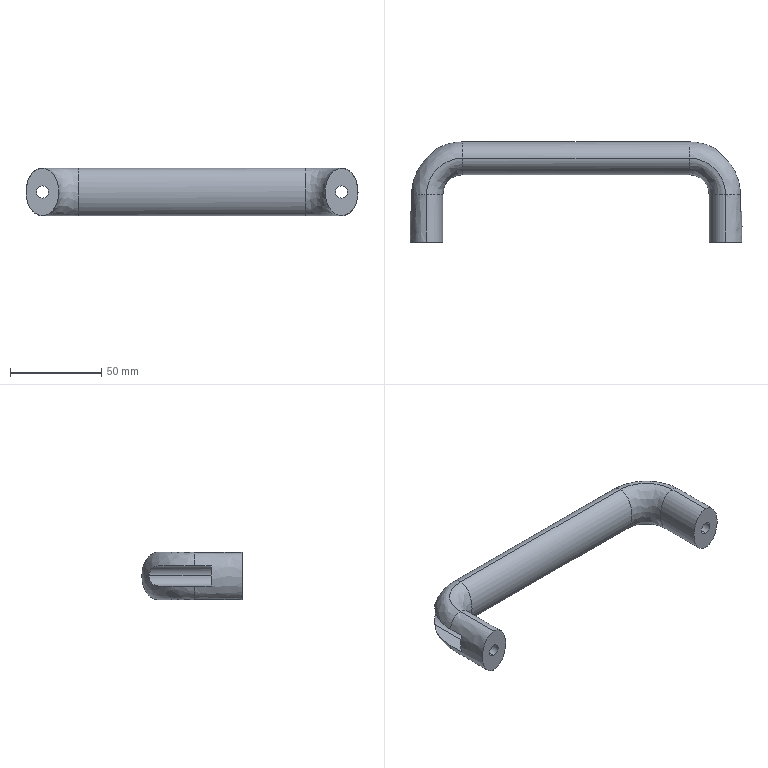Part | SolidWorks | features BaseBody 1 | 1 solid | 28 faces | box 182 x 55 x 26 mm | volume 78425 mm3 | plane 10 | spline 10 | cylinder 8 | commonest cylinder face diameters 6.6 x4 11 x4
STEP:
#1=CARTESIAN_POINT('',(76.5,51.115,0.));
#2=VERTEX_POINT('',#1);
#3=CARTESIAN_POINT('',(82.,45.817,-5.5));
#4=VERTEX_POINT('',#3);
#5=CARTESIAN_POINT('',(76.5,51.115,0.));
#6=CARTESIAN_POINT('',(76.5,51.115,-0.4392));
#7=CARTESIAN_POINT('',(76.552,51.067,-0.8654));
#8=CARTESIAN_POINT('',(76.701,50.931,-1.487));
#9=CARTESIAN_POINT('',(76.762,50.874,-1.691));
#10=CARTESIAN_POINT('',(76.904,50.743,-2.079));
#11=CARTESIAN_POINT('',(76.985,50.669,-2.266));
#12=CARTESIAN_POINT('',(77.163,50.504,-2.626));
#13=CARTESIAN_POINT('',(77.262,50.412,-2.8));
#14=CARTESIAN_POINT('',(77.471,50.217,-3.127));
#15=CARTESIAN_POINT('',(77.582,50.113,-3.281));
#16=CARTESIAN_POINT('',(77.814,49.895,-3.573));
#17=CARTESIAN_POINT('',(77.936,49.781,-3.71));
#18=CARTESIAN_POINT('',(78.188,49.543,-3.969));
#19=CARTESIAN_POINT('',(78.32,49.418,-4.091));
#20=CARTESIAN_POINT('',(78.993,48.778,-4.659));
#21=CARTESIAN_POINT('',(79.57,48.222,-4.975));
#22=CARTESIAN_POINT('',(80.778,47.04,-5.401));
#23=CARTESIAN_POINT('',(81.387,46.435,-5.5));
#24=CARTESIAN_POINT('',(82.,45.817,-5.5));
#25=B_SPLINE_CURVE_WITH_KNOTS('',3,(#5,#6,#7,#8,#9,#10,#11,#12,#13,#14,#15,#16,#17,#18,#19,#20,#21,#22,#23,#24),.UNSPECIFIED.,.F.,.F.,(4,2,2,2,2,2,2,2,2,4),(0.,0.001296,0.001943,0.002591,0.003239,0.003887,0.004535,0.005182,0.007774,0.01036),.UNSPECIFIED.);
#26=EDGE_CURVE('',#2,#4,#25,.T.);
#27=ORIENTED_EDGE('',*,*,#26,.F.);
#28=CARTESIAN_POINT('',(76.5,11.,0.));
#29=VERTEX_POINT('',#28);
#30=CARTESIAN_POINT('',(76.5,55.,0.));
#31=DIRECTION('',(0.,-1.,0.));
#32=VECTOR('',#31,1000.);
#33=LINE('',#30,#32);
#34=EDGE_CURVE('',#2,#29,#33,.T.);
#35=ORIENTED_EDGE('',*,*,#34,.T.);
#36=CARTESIAN_POINT('',(87.5,11.,0.));
#37=VERTEX_POINT('',#36);
#38=CARTESIAN_POINT('',(82.,11.,0.));
#39=DIRECTION('',(0.,1.,0.));
#40=DIRECTION('',(1.,0.,0.));
#41=AXIS2_PLACEMENT_3D('',#38,#39,#40);
#42=CIRCLE('',#41,5.5);
#43=EDGE_CURVE('',#37,#29,#42,.T.);
#44=ORIENTED_EDGE('',*,*,#43,.F.);
#45=CARTESIAN_POINT('',(87.5,17.,0.));
#46=VERTEX_POINT('',#45);
#47=CARTESIAN_POINT('',(87.5,55.,0.));
#48=DIRECTION('',(0.,-1.,0.));
#49=VECTOR('',#48,1000.);
#50=LINE('',#47,#49);
#51=EDGE_CURVE('',#46,#37,#50,.T.);
#52=ORIENTED_EDGE('',*,*,#51,.F.);
#53=CARTESIAN_POINT('',(82.,17.,-5.5));
#54=VERTEX_POINT('',#53);
#55=CARTESIAN_POINT('',(82.,17.,0.));
#56=DIRECTION('',(0.,-1.,0.));
#57=DIRECTION('',(1.,0.,0.));
#58=AXIS2_PLACEMENT_3D('',#55,#56,#57);
#59=CIRCLE('',#58,5.5);
#60=EDGE_CURVE('',#54,#46,#59,.T.);
#61=ORIENTED_EDGE('',*,*,#60,.F.);
#62=CARTESIAN_POINT('',(82.,55.,-5.5));
#63=DIRECTION('',(0.,-1.,0.));
#64=VECTOR('',#63,1000.);
#65=LINE('',#62,#64);
#66=EDGE_CURVE('',#4,#54,#65,.T.);
#67=ORIENTED_EDGE('',*,*,#66,.F.);
#68=EDGE_LOOP('',(#27,#35,#44,#52,#61,#67));
#69=FACE_OUTER_BOUND('',#68,.T.);
#70=CARTESIAN_POINT('',(82.,55.,0.));
#71=DIRECTION('',(0.,-1.,0.));
#72=DIRECTION('',(1.,0.,0.));
#73=AXIS2_PLACEMENT_3D('',#70,#71,#72);
#74=CYLINDRICAL_SURFACE('',#73,5.5);
#75=ADVANCED_FACE('',(#69),#74,.F.);
#76=CARTESIAN_POINT('',(-87.5,17.,0.));
#77=VERTEX_POINT('',#76);
#78=CARTESIAN_POINT('',(-82.,17.,-5.5));
#79=VERTEX_POINT('',#78);
#80=CARTESIAN_POINT('',(-82.,17.,0.));
#81=DIRECTION('',(0.,-1.,0.));
#82=DIRECTION('',(1.,0.,0.));
#83=AXIS2_PLACEMENT_3D('',#80,#81,#82);
#84=CIRCLE('',#83,5.5);
#85=EDGE_CURVE('',#77,#79,#84,.T.);
#86=ORIENTED_EDGE('',*,*,#85,.F.);
#87=CARTESIAN_POINT('',(-87.5,11.,0.));
#88=VERTEX_POINT('',#87);
#89=CARTESIAN_POINT('',(-87.5,55.,0.));
#90=DIRECTION('',(0.,-1.,0.));
#91=VECTOR('',#90,1000.);
#92=LINE('',#89,#91);
#93=EDGE_CURVE('',#77,#88,#92,.T.);
#94=ORIENTED_EDGE('',*,*,#93,.T.);
#95=CARTESIAN_POINT('',(-76.5,11.,0.));
#96=VERTEX_POINT('',#95);
#97=CARTESIAN_POINT('',(-82.,11.,0.));
#98=DIRECTION('',(0.,1.,0.));
#99=DIRECTION('',(1.,0.,0.));
#100=AXIS2_PLACEMENT_3D('',#97,#98,#99);
#101=CIRCLE('',#100,5.5);
#102=EDGE_CURVE('',#96,#88,#101,.T.);
#103=ORIENTED_EDGE('',*,*,#102,.F.);
#104=CARTESIAN_POINT('',(-76.5,51.115,0.));
#105=VERTEX_POINT('',#104);
#106=CARTESIAN_POINT('',(-76.5,55.,0.));
#107=DIRECTION('',(0.,-1.,0.));
#108=VECTOR('',#107,1000.);
#109=LINE('',#106,#108);
#110=EDGE_CURVE('',#105,#96,#109,.T.);
#111=ORIENTED_EDGE('',*,*,#110,.F.);
#112=CARTESIAN_POINT('',(-82.,45.817,-5.5));
#113=VERTEX_POINT('',#112);
#114=CARTESIAN_POINT('',(-82.,45.817,-5.5));
#115=CARTESIAN_POINT('',(-81.387,46.435,-5.5));
#116=CARTESIAN_POINT('',(-80.781,47.037,-5.4));
#117=CARTESIAN_POINT('',(-79.885,47.914,-5.087));
#118=CARTESIAN_POINT('',(-79.586,48.204,-4.953));
#119=CARTESIAN_POINT('',(-79.007,48.763,-4.626));
#120=CARTESIAN_POINT('',(-78.728,49.03,-4.435));
#121=CARTESIAN_POINT('',(-78.193,49.539,-3.985));
#122=CARTESIAN_POINT('',(-77.935,49.782,-3.723));
#123=CARTESIAN_POINT('',(-77.468,50.22,-3.139));
#124=CARTESIAN_POINT('',(-77.258,50.416,-2.815));
#125=CARTESIAN_POINT('',(-76.897,50.75,-2.09));
#126=CARTESIAN_POINT('',(-76.753,50.883,-1.703));
#127=CARTESIAN_POINT('',(-76.603,51.02,-1.082));
#128=CARTESIAN_POINT('',(-76.564,51.056,-0.8672));
#129=CARTESIAN_POINT('',(-76.513,51.103,-0.437));
#130=CARTESIAN_POINT('',(-76.5,51.115,-0.2197));
#131=CARTESIAN_POINT('',(-76.5,51.115,0.));
#132=B_SPLINE_CURVE_WITH_KNOTS('',3,(#114,#115,#116,#117,#118,#119,#120,#121,#122,#123,#124,#125,#126,#127,#128,#129,#130,#131),.UNSPECIFIED.,.F.,.F.,(4,2,2,2,2,2,2,2,4),(0.,0.002576,0.003865,0.005153,0.006441,0.007729,0.009018,0.009662,0.01031),.UNSPECIFIED.);
#133=EDGE_CURVE('',#113,#105,#132,.T.);
#134=ORIENTED_EDGE('',*,*,#133,.F.);
#135=CARTESIAN_POINT('',(-82.,55.,-5.5));
#136=DIRECTION('',(0.,1.,0.));
#137=VECTOR('',#136,1000.);
#138=LINE('',#135,#137);
#139=EDGE_CURVE('',#79,#113,#138,.T.);
#140=ORIENTED_EDGE('',*,*,#139,.F.);
#141=EDGE_LOOP('',(#86,#94,#103,#111,#134,#140));
#142=FACE_OUTER_BOUND('',#141,.T.);
#143=CARTESIAN_POINT('',(-82.,55.,0.));
#144=DIRECTION('',(0.,-1.,0.));
#145=DIRECTION('',(1.,0.,0.));
#146=AXIS2_PLACEMENT_3D('',#143,#144,#145);
#147=CYLINDRICAL_SURFACE('',#146,5.5);
#148=ADVANCED_FACE('',(#142),#147,.F.);
#149=CARTESIAN_POINT('',(82.,0.,-3.3));
#150=VERTEX_POINT('',#149);
#151=CARTESIAN_POINT('',(82.,0.,3.3));
#152=VERTEX_POINT('',#151);
#153=CARTESIAN_POINT('',(82.,0.,0.));
#154=DIRECTION('',(0.,1.,0.));
#155=DIRECTION('',(0.,0.,1.));
#156=AXIS2_PLACEMENT_3D('',#153,#154,#155);
#157=CIRCLE('',#156,3.3);
#158=EDGE_CURVE('',#150,#152,#157,.T.);
#159=ORIENTED_EDGE('',*,*,#158,.F.);
#160=CARTESIAN_POINT('',(82.,11.,-3.3));
#161=VERTEX_POINT('',#160);
#162=CARTESIAN_POINT('',(82.,17.,-3.3));
#163=DIRECTION('',(0.,1.,0.));
#164=VECTOR('',#163,1000.);
#165=LINE('',#162,#164);
#166=EDGE_CURVE('',#150,#161,#165,.T.);
#167=ORIENTED_EDGE('',*,*,#166,.T.);
#168=CARTESIAN_POINT('',(82.,11.,3.3));
#169=VERTEX_POINT('',#168);
#170=CARTESIAN_POINT('',(82.,11.,0.));
#171=DIRECTION('',(0.,1.,0.));
#172=DIRECTION('',(0.,0.,1.));
#173=AXIS2_PLACEMENT_3D('',#170,#171,#172);
#174=CIRCLE('',#173,3.3);
#175=EDGE_CURVE('',#161,#169,#174,.T.);
#176=ORIENTED_EDGE('',*,*,#175,.T.);
#177=CARTESIAN_POINT('',(82.,17.,3.3));
#178=DIRECTION('',(0.,1.,0.));
#179=VECTOR('',#178,1000.);
#180=LINE('',#177,#179);
#181=EDGE_CURVE('',#152,#169,#180,.T.);
#182=ORIENTED_EDGE('',*,*,#181,.F.);
#183=EDGE_LOOP('',(#159,#167,#176,#182));
#184=FACE_OUTER_BOUND('',#183,.T.);
#185=CARTESIAN_POINT('',(82.,17.,0.));
#186=DIRECTION('',(0.,1.,0.));
#187=DIRECTION('',(0.,0.,1.));
#188=AXIS2_PLACEMENT_3D('',#185,#186,#187);
#189=CYLINDRICAL_SURFACE('',#188,3.3);
#190=ADVANCED_FACE('',(#184),#189,.F.);
#191=CARTESIAN_POINT('',(-82.,0.,3.3));
#192=VERTEX_POINT('',#191);
#193=CARTESIAN_POINT('',(-82.,0.,-3.3));
#194=VERTEX_POINT('',#193);
#195=CARTESIAN_POINT('',(-82.,0.,0.));
#196=DIRECTION('',(0.,-1.,0.));
#197=DIRECTION('',(0.,0.,1.));
#198=AXIS2_PLACEMENT_3D('',#195,#196,#197);
#199=CIRCLE('',#198,3.3);
#200=EDGE_CURVE('',#192,#194,#199,.T.);
#201=ORIENTED_EDGE('',*,*,#200,.T.);
#202=CARTESIAN_POINT('',(-82.,11.,-3.3));
#203=VERTEX_POINT('',#202);
#204=CARTESIAN_POINT('',(-82.,17.,-3.3));
#205=DIRECTION('',(0.,1.,0.));
#206=VECTOR('',#205,1000.);
#207=LINE('',#204,#206);
#208=EDGE_CURVE('',#194,#203,#207,.T.);
#209=ORIENTED_EDGE('',*,*,#208,.T.);
#210=CARTESIAN_POINT('',(-82.,11.,3.3));
#211=VERTEX_POINT('',#210);
#212=CARTESIAN_POINT('',(-82.,11.,0.));
#213=DIRECTION('',(0.,1.,0.));
#214=DIRECTION('',(0.,0.,1.));
#215=AXIS2_PLACEMENT_3D('',#212,#213,#214);
#216=CIRCLE('',#215,3.3);
#217=EDGE_CURVE('',#203,#211,#216,.T.);
#218=ORIENTED_EDGE('',*,*,#217,.T.);
#219=CARTESIAN_POINT('',(-82.,17.,3.3));
#220=DIRECTION('',(0.,1.,0.));
#221=VECTOR('',#220,1000.);
#222=LINE('',#219,#221);
#223=EDGE_CURVE('',#192,#211,#222,.T.);
#224=ORIENTED_EDGE('',*,*,#223,.F.);
#225=EDGE_LOOP('',(#201,#209,#218,#224));
#226=FACE_OUTER_BOUND('',#225,.T.);
#227=CARTESIAN_POINT('',(-82.,17.,0.));
#228=DIRECTION('',(0.,1.,0.));
#229=DIRECTION('',(0.,0.,1.));
#230=AXIS2_PLACEMENT_3D('',#227,#228,#229);
#231=CYLINDRICAL_SURFACE('',#230,3.3);
#232=ADVANCED_FACE('',(#226),#231,.F.);
#233=ORIENTED_EDGE('',*,*,#200,.F.);
#234=CARTESIAN_POINT('',(-82.,0.,0.));
#235=DIRECTION('',(0.,-1.,0.));
#236=DIRECTION('',(0.,0.,1.));
#237=AXIS2_PLACEMENT_3D('',#234,#235,#236);
#238=CIRCLE('',#237,3.3);
#239=EDGE_CURVE('',#194,#192,#238,.T.);
#240=ORIENTED_EDGE('',*,*,#239,.F.);
#241=EDGE_LOOP('',(#233,#240));
#242=FACE_BOUND('',#241,.T.);
#243=CARTESIAN_POINT('',(-82.,0.,-13.));
#244=VERTEX_POINT('',#243);
#245=CARTESIAN_POINT('',(-82.,0.,13.));
#246=VERTEX_POINT('',#245);
#247=CARTESIAN_POINT('',(-82.,0.,-13.));
#248=CARTESIAN_POINT('',(-64.,0.,-13.));
#249=CARTESIAN_POINT('',(-64.,0.,13.));
#250=CARTESIAN_POINT('',(-82.,0.,13.));
#251=(BOUNDED_CURVE()B_SPLINE_CURVE(3,(#247,#248,#249,#250),.UNSPECIFIED.,.F.,.F.)B_SPLINE_CURVE_WITH_KNOTS((4,4),(0.,0.0348),.UNSPECIFIED.)CURVE()GEOMETRIC_REPRESENTATION_ITEM()RATIONAL_B_SPLINE_CURVE((1.,0.3333,0.3333,1.))REPRESENTATION_ITEM(''));
#252=EDGE_CURVE('',#244,#246,#251,.T.);
#253=ORIENTED_EDGE('',*,*,#252,.T.);
#254=CARTESIAN_POINT('',(-82.,0.,13.));
#255=CARTESIAN_POINT('',(-100.,0.,13.));
#256=CARTESIAN_POINT('',(-100.,0.,-13.));
#257=CARTESIAN_POINT('',(-82.,0.,-13.));
#258=(BOUNDED_CURVE()B_SPLINE_CURVE(3,(#254,#255,#256,#257),.UNSPECIFIED.,.F.,.T.)B_SPLINE_CURVE_WITH_KNOTS((4,4),(0.,0.0348),.UNSPECIFIED.)CURVE()GEOMETRIC_REPRESENTATION_ITEM()RATIONAL_B_SPLINE_CURVE((1.,0.3333,0.3333,1.))REPRESENTATION_ITEM(''));
#259=EDGE_CURVE('',#246,#244,#258,.T.);
#260=ORIENTED_EDGE('',*,*,#259,.T.);
#261=EDGE_LOOP('',(#253,#260));
#262=FACE_OUTER_BOUND('',#261,.T.);
#263=CARTESIAN_POINT('',(-82.,0.,0.));
#264=DIRECTION('',(0.,1.,0.));
#265=DIRECTION('',(1.,0.,0.));
#266=AXIS2_PLACEMENT_3D('',#263,#264,#265);
#267=PLANE('',#266);
#268=ADVANCED_FACE('',(#242,#262),#267,.F.);
#269=CARTESIAN_POINT('',(-82.,11.,0.));
#270=DIRECTION('',(0.,1.,0.));
#271=DIRECTION('',(0.,0.,1.));
#272=AXIS2_PLACEMENT_3D('',#269,#270,#271);
#273=CIRCLE('',#272,3.3);
#274=EDGE_CURVE('',#211,#203,#273,.T.);
#275=ORIENTED_EDGE('',*,*,#274,.F.);
#276=ORIENTED_EDGE('',*,*,#217,.F.);
#277=EDGE_LOOP('',(#275,#276));
#278=FACE_BOUND('',#277,.T.);
#279=ORIENTED_EDGE('',*,*,#102,.T.);
#280=CARTESIAN_POINT('',(-82.,11.,0.));
#281=DIRECTION('',(0.,1.,0.));
#282=DIRECTION('',(1.,0.,0.));
#283=AXIS2_PLACEMENT_3D('',#280,#281,#282);
#284=CIRCLE('',#283,5.5);
#285=EDGE_CURVE('',#88,#96,#284,.T.);
#286=ORIENTED_EDGE('',*,*,#285,.T.);
#287=EDGE_LOOP('',(#279,#286));
#288=FACE_OUTER_BOUND('',#287,.T.);
#289=CARTESIAN_POINT('',(-78.7,11.,0.));
#290=DIRECTION('',(0.,-1.,0.));
#291=DIRECTION('',(0.,0.,-1.));
#292=AXIS2_PLACEMENT_3D('',#289,#290,#291);
#293=PLANE('',#292);
#294=ADVANCED_FACE('',(#278,#288),#293,.F.);
#295=CARTESIAN_POINT('',(-90.155,17.,5.5));
#296=VERTEX_POINT('',#295);
#297=CARTESIAN_POINT('',(-82.,17.,5.5));
#298=VERTEX_POINT('',#297);
#299=CARTESIAN_POINT('',(-82.,17.,5.5));
#300=DIRECTION('',(1.,0.,0.));
#301=VECTOR('',#300,1000.);
#302=LINE('',#299,#301);
#303=EDGE_CURVE('',#296,#298,#302,.T.);
#304=ORIENTED_EDGE('',*,*,#303,.T.);
#305=CARTESIAN_POINT('',(-82.,17.,0.));
#306=DIRECTION('',(0.,-1.,0.));
#307=DIRECTION('',(1.,0.,0.));
#308=AXIS2_PLACEMENT_3D('',#305,#306,#307);
#309=CIRCLE('',#308,5.5);
#310=EDGE_CURVE('',#298,#77,#309,.T.);
#311=ORIENTED_EDGE('',*,*,#310,.T.);
#312=ORIENTED_EDGE('',*,*,#85,.T.);
#313=CARTESIAN_POINT('',(-90.155,17.,-5.5));
#314=VERTEX_POINT('',#313);
#315=CARTESIAN_POINT('',(-82.,17.,-5.5));
#316=DIRECTION('',(-1.,0.,0.));
#317=VECTOR('',#316,1000.);
#318=LINE('',#315,#317);
#319=EDGE_CURVE('',#79,#314,#318,.T.);
#320=ORIENTED_EDGE('',*,*,#319,.T.);
#321=CARTESIAN_POINT('',(-90.155,17.,-5.5));
#322=CARTESIAN_POINT('',(-91.301,17.,-1.956));
#323=CARTESIAN_POINT('',(-91.301,17.,1.956));
#324=CARTESIAN_POINT('',(-90.155,17.,5.5));
#325=(BOUNDED_CURVE()B_SPLINE_CURVE(3,(#321,#322,#323,#324),.UNSPECIFIED.,.F.,.T.)B_SPLINE_CURVE_WITH_KNOTS((4,4),(0.,0.01112),.UNSPECIFIED.)CURVE()GEOMETRIC_REPRESENTATION_ITEM()RATIONAL_B_SPLINE_CURVE((0.5246,0.4918,0.4918,0.5246))REPRESENTATION_ITEM(''));
#326=EDGE_CURVE('',#314,#296,#325,.T.);
#327=ORIENTED_EDGE('',*,*,#326,.T.);
#328=EDGE_LOOP('',(#304,#311,#312,#320,#327));
#329=FACE_OUTER_BOUND('',#328,.T.);
#330=CARTESIAN_POINT('',(-82.,17.,0.));
#331=DIRECTION('',(0.,-1.,0.));
#332=DIRECTION('',(-1.,0.,0.));
#333=AXIS2_PLACEMENT_3D('',#330,#331,#332);
#334=PLANE('',#333);
#335=ADVANCED_FACE('',(#329),#334,.F.);
#336=CARTESIAN_POINT('',(82.,11.,0.));
#337=DIRECTION('',(0.,1.,0.));
#338=DIRECTION('',(0.,0.,1.));
#339=AXIS2_PLACEMENT_3D('',#336,#337,#338);
#340=CIRCLE('',#339,3.3);
#341=EDGE_CURVE('',#169,#161,#340,.T.);
#342=ORIENTED_EDGE('',*,*,#341,.F.);
#343=ORIENTED_EDGE('',*,*,#175,.F.);
#344=EDGE_LOOP('',(#342,#343));
#345=FACE_BOUND('',#344,.T.);
#346=ORIENTED_EDGE('',*,*,#43,.T.);
#347=CARTESIAN_POINT('',(82.,11.,0.));
#348=DIRECTION('',(0.,1.,0.));
#349=DIRECTION('',(1.,0.,0.));
#350=AXIS2_PLACEMENT_3D('',#347,#348,#349);
#351=CIRCLE('',#350,5.5);
#352=EDGE_CURVE('',#29,#37,#351,.T.);
#353=ORIENTED_EDGE('',*,*,#352,.T.);
#354=EDGE_LOOP('',(#346,#353));
#355=FACE_OUTER_BOUND('',#354,.T.);
#356=CARTESIAN_POINT('',(85.3,11.,0.));
#357=DIRECTION('',(0.,-1.,0.));
#358=DIRECTION('',(0.,0.,-1.));
#359=AXIS2_PLACEMENT_3D('',#356,#357,#358);
#360=PLANE('',#359);
#361=ADVANCED_FACE('',(#345,#355),#360,.F.);
#362=CARTESIAN_POINT('',(82.,0.,0.));
#363=DIRECTION('',(0.,1.,0.));
#364=DIRECTION('',(0.,0.,1.));
#365=AXIS2_PLACEMENT_3D('',#362,#363,#364);
#366=CIRCLE('',#365,3.3);
#367=EDGE_CURVE('',#152,#150,#366,.T.);
#368=ORIENTED_EDGE('',*,*,#367,.T.);
#369=ORIENTED_EDGE('',*,*,#158,.T.);
#370=EDGE_LOOP('',(#368,#369));
#371=FACE_BOUND('',#370,.T.);
#372=CARTESIAN_POINT('',(82.,0.,13.));
#373=VERTEX_POINT('',#372);
#374=CARTESIAN_POINT('',(82.,0.,-13.));
#375=VERTEX_POINT('',#374);
#376=CARTESIAN_POINT('',(82.,0.,13.));
#377=CARTESIAN_POINT('',(100.,0.,13.));
#378=CARTESIAN_POINT('',(100.,0.,-13.));
#379=CARTESIAN_POINT('',(82.,0.,-13.));
#380=(BOUNDED_CURVE()B_SPLINE_CURVE(3,(#376,#377,#378,#379),.UNSPECIFIED.,.F.,.F.)B_SPLINE_CURVE_WITH_KNOTS((4,4),(0.,0.0348),.UNSPECIFIED.)CURVE()GEOMETRIC_REPRESENTATION_ITEM()RATIONAL_B_SPLINE_CURVE((1.,0.3333,0.3333,1.))REPRESENTATION_ITEM(''));
#381=EDGE_CURVE('',#373,#375,#380,.T.);
#382=ORIENTED_EDGE('',*,*,#381,.F.);
#383=CARTESIAN_POINT('',(82.,0.,-13.));
#384=CARTESIAN_POINT('',(64.,0.,-13.));
#385=CARTESIAN_POINT('',(64.,0.,13.));
#386=CARTESIAN_POINT('',(82.,0.,13.));
#387=(BOUNDED_CURVE()B_SPLINE_CURVE(3,(#383,#384,#385,#386),.UNSPECIFIED.,.F.,.T.)B_SPLINE_CURVE_WITH_KNOTS((4,4),(0.,0.0348),.UNSPECIFIED.)CURVE()GEOMETRIC_REPRESENTATION_ITEM()RATIONAL_B_SPLINE_CURVE((1.,0.3333,0.3333,1.))REPRESENTATION_ITEM(''));
#388=EDGE_CURVE('',#375,#373,#387,.T.);
#389=ORIENTED_EDGE('',*,*,#388,.F.);
#390=EDGE_LOOP('',(#382,#389));
#391=FACE_OUTER_BOUND('',#390,.T.);
#392=CARTESIAN_POINT('',(82.,0.,0.));
#393=DIRECTION('',(0.,-1.,0.));
#394=DIRECTION('',(-1.,0.,0.));
#395=AXIS2_PLACEMENT_3D('',#392,#393,#394);
#396=PLANE('',#395);
#397=ADVANCED_FACE('',(#371,#391),#396,.T.);
#398=ORIENTED_EDGE('',*,*,#60,.T.);
#399=CARTESIAN_POINT('',(82.,17.,5.5));
#400=VERTEX_POINT('',#399);
#401=CARTESIAN_POINT('',(82.,17.,0.));
#402=DIRECTION('',(0.,-1.,0.));
#403=DIRECTION('',(1.,0.,0.));
#404=AXIS2_PLACEMENT_3D('',#401,#402,#403);
#405=CIRCLE('',#404,5.5);
#406=EDGE_CURVE('',#46,#400,#405,.T.);
#407=ORIENTED_EDGE('',*,*,#406,.T.);
#408=CARTESIAN_POINT('',(90.155,17.,5.5));
#409=VERTEX_POINT('',#408);
#410=CARTESIAN_POINT('',(82.,17.,5.5));
#411=DIRECTION('',(-1.,0.,0.));
#412=VECTOR('',#411,1000.);
#413=LINE('',#410,#412);
#414=EDGE_CURVE('',#409,#400,#413,.T.);
#415=ORIENTED_EDGE('',*,*,#414,.F.);
#416=CARTESIAN_POINT('',(90.155,17.,-5.5));
#417=VERTEX_POINT('',#416);
#418=CARTESIAN_POINT('',(90.155,17.,-5.5));
#419=CARTESIAN_POINT('',(91.301,17.,-1.956));
#420=CARTESIAN_POINT('',(91.301,17.,1.956));
#421=CARTESIAN_POINT('',(90.155,17.,5.5));
#422=(BOUNDED_CURVE()B_SPLINE_CURVE(3,(#418,#419,#420,#421),.UNSPECIFIED.,.F.,.F.)B_SPLINE_CURVE_WITH_KNOTS((4,4),(0.,0.01112),.UNSPECIFIED.)CURVE()GEOMETRIC_REPRESENTATION_ITEM()RATIONAL_B_SPLINE_CURVE((0.5246,0.4918,0.4918,0.5246))REPRESENTATION_ITEM(''));
#423=EDGE_CURVE('',#417,#409,#422,.T.);
#424=ORIENTED_EDGE('',*,*,#423,.F.);
#425=CARTESIAN_POINT('',(82.,17.,-5.5));
#426=DIRECTION('',(1.,0.,0.));
#427=VECTOR('',#426,1000.);
#428=LINE('',#425,#427);
#429=EDGE_CURVE('',#54,#417,#428,.T.);
#430=ORIENTED_EDGE('',*,*,#429,.F.);
#431=EDGE_LOOP('',(#398,#407,#415,#424,#430));
#432=FACE_OUTER_BOUND('',#431,.T.);
#433=CARTESIAN_POINT('',(82.,17.,0.));
#434=DIRECTION('',(0.,-1.,0.));
#435=DIRECTION('',(0.,0.,-1.));
#436=AXIS2_PLACEMENT_3D('',#433,#434,#435);
#437=PLANE('',#436);
#438=ADVANCED_FACE('',(#432),#437,.F.);
#439=CARTESIAN_POINT('',(-82.,26.,13.));
#440=VERTEX_POINT('',#439);
#441=CARTESIAN_POINT('',(-82.,13.,13.));
#442=DIRECTION('',(0.,-1.,0.));
#443=VECTOR('',#442,1000.);
#444=LINE('',#441,#443);
#445=EDGE_CURVE('',#440,#246,#444,.T.);
#446=ORIENTED_EDGE('',*,*,#445,.T.);
#447=ORIENTED_EDGE('',*,*,#252,.F.);
#448=CARTESIAN_POINT('',(-82.,26.,-13.));
#449=VERTEX_POINT('',#448);
#450=CARTESIAN_POINT('',(-82.,13.,-13.));
#451=DIRECTION('',(0.,1.,0.));
#452=VECTOR('',#451,1000.);
#453=LINE('',#450,#452);
#454=EDGE_CURVE('',#244,#449,#453,.T.);
#455=ORIENTED_EDGE('',*,*,#454,.T.);
#456=CARTESIAN_POINT('',(-82.,26.,13.));
#457=CARTESIAN_POINT('',(-64.,26.,13.));
#458=CARTESIAN_POINT('',(-64.,26.,-13.));
#459=CARTESIAN_POINT('',(-82.,26.,-13.));
#460=(BOUNDED_CURVE()B_SPLINE_CURVE(3,(#456,#457,#458,#459),.UNSPECIFIED.,.F.,.F.)B_SPLINE_CURVE_WITH_KNOTS((4,4),(0.,1.),.UNSPECIFIED.)CURVE()GEOMETRIC_REPRESENTATION_ITEM()RATIONAL_B_SPLINE_CURVE((1.,0.3333,0.3333,1.))REPRESENTATION_ITEM(''));
#461=EDGE_CURVE('',#440,#449,#460,.T.);
#462=ORIENTED_EDGE('',*,*,#461,.F.);
#463=EDGE_LOOP('',(#446,#447,#455,#462));
#464=FACE_OUTER_BOUND('',#463,.T.);
#465=CARTESIAN_POINT('',(-82.,26.,13.));
#466=CARTESIAN_POINT('',(-82.,0.,13.));
#467=CARTESIAN_POINT('',(-64.,26.,13.));
#468=CARTESIAN_POINT('',(-64.,0.,13.));
#469=CARTESIAN_POINT('',(-64.,26.,-13.));
#470=CARTESIAN_POINT('',(-64.,0.,-13.));
#471=CARTESIAN_POINT('',(-82.,26.,-13.));
#472=CARTESIAN_POINT('',(-82.,0.,-13.));
#473=(BOUNDED_SURFACE()B_SPLINE_SURFACE(3,1,((#465,#466),(#467,#468),(#469,#470),(#471,#472)),.UNSPECIFIED.,.F.,.F.,.T.)B_SPLINE_SURFACE_WITH_KNOTS((4,4),(2,2),(0.,1.),(0.,1.),.UNSPECIFIED.)GEOMETRIC_REPRESENTATION_ITEM()RATIONAL_B_SPLINE_SURFACE(((1.,1.),(0.3333,0.3333),(0.3333,0.3333),(1.,1.)))REPRESENTATION_ITEM('')SURFACE());
#474=ADVANCED_FACE('',(#464),#473,.F.);
#475=CARTESIAN_POINT('',(82.,26.,-13.));
#476=VERTEX_POINT('',#475);
#477=CARTESIAN_POINT('',(82.,13.,-13.));
#478=DIRECTION('',(0.,1.,0.));
#479=VECTOR('',#478,1000.);
#480=LINE('',#477,#479);
#481=EDGE_CURVE('',#375,#476,#480,.T.);
#482=ORIENTED_EDGE('',*,*,#481,.F.);
#483=ORIENTED_EDGE('',*,*,#388,.T.);
#484=CARTESIAN_POINT('',(82.,26.,13.));
#485=VERTEX_POINT('',#484);
#486=CARTESIAN_POINT('',(82.,13.,13.));
#487=DIRECTION('',(0.,-1.,0.));
#488=VECTOR('',#487,1000.);
#489=LINE('',#486,#488);
#490=EDGE_CURVE('',#485,#373,#489,.T.);
#491=ORIENTED_EDGE('',*,*,#490,.F.);
#492=CARTESIAN_POINT('',(82.,26.,-13.));
#493=CARTESIAN_POINT('',(64.,26.,-13.));
#494=CARTESIAN_POINT('',(64.,26.,13.));
#495=CARTESIAN_POINT('',(82.,26.,13.));
#496=(BOUNDED_CURVE()B_SPLINE_CURVE(3,(#492,#493,#494,#495),.UNSPECIFIED.,.F.,.T.)B_SPLINE_CURVE_WITH_KNOTS((4,4),(0.,1.),.UNSPECIFIED.)CURVE()GEOMETRIC_REPRESENTATION_ITEM()RATIONAL_B_SPLINE_CURVE((1.,0.3333,0.3333,1.))REPRESENTATION_ITEM(''));
#497=EDGE_CURVE('',#476,#485,#496,.T.);
#498=ORIENTED_EDGE('',*,*,#497,.F.);
#499=EDGE_LOOP('',(#482,#483,#491,#498));
#500=FACE_OUTER_BOUND('',#499,.T.);
#501=CARTESIAN_POINT('',(82.,26.,13.));
#502=CARTESIAN_POINT('',(82.,0.,13.));
#503=CARTESIAN_POINT('',(64.,26.,13.));
#504=CARTESIAN_POINT('',(64.,0.,13.));
#505=CARTESIAN_POINT('',(64.,26.,-13.));
#506=CARTESIAN_POINT('',(64.,0.,-13.));
#507=CARTESIAN_POINT('',(82.,26.,-13.));
#508=CARTESIAN_POINT('',(82.,0.,-13.));
#509=(BOUNDED_SURFACE()B_SPLINE_SURFACE(3,1,((#501,#502),(#503,#504),(#505,#506),(#507,#508)),.UNSPECIFIED.,.F.,.F.,.T.)B_SPLINE_SURFACE_WITH_KNOTS((4,4),(2,2),(0.,1.),(0.,1.),.UNSPECIFIED.)GEOMETRIC_REPRESENTATION_ITEM()RATIONAL_B_SPLINE_SURFACE(((1.,1.),(0.3333,0.3333),(0.3333,0.3333),(1.,1.)))REPRESENTATION_ITEM('')SURFACE());
#510=ADVANCED_FACE('',(#500),#509,.T.);
#511=CARTESIAN_POINT('',(-90.155,26.,5.5));
#512=VERTEX_POINT('',#511);
#513=CARTESIAN_POINT('',(-90.155,26.,5.5));
#514=CARTESIAN_POINT('',(-88.459,26.,10.747));
#515=CARTESIAN_POINT('',(-85.151,26.,13.));
#516=CARTESIAN_POINT('',(-82.,26.,13.));
#517=(BOUNDED_CURVE()B_SPLINE_CURVE(3,(#513,#514,#515,#516),.UNSPECIFIED.,.F.,.F.)B_SPLINE_CURVE_WITH_KNOTS((4,4),(0.611,1.),.UNSPECIFIED.)CURVE()GEOMETRIC_REPRESENTATION_ITEM()RATIONAL_B_SPLINE_CURVE((0.5246,0.5822,0.7407,1.))REPRESENTATION_ITEM(''));
#518=EDGE_CURVE('',#512,#440,#517,.T.);
#519=ORIENTED_EDGE('',*,*,#518,.F.);
#520=CARTESIAN_POINT('',(-90.155,55.,5.5));
#521=DIRECTION('',(0.,-1.,0.));
#522=VECTOR('',#521,1000.);
#523=LINE('',#520,#522);
#524=EDGE_CURVE('',#512,#296,#523,.T.);
#525=ORIENTED_EDGE('',*,*,#524,.T.);
#526=ORIENTED_EDGE('',*,*,#326,.F.);
#527=CARTESIAN_POINT('',(-90.155,26.,-5.5));
#528=VERTEX_POINT('',#527);
#529=CARTESIAN_POINT('',(-90.155,55.,-5.5));
#530=DIRECTION('',(0.,1.,0.));
#531=VECTOR('',#530,1000.);
#532=LINE('',#529,#531);
#533=EDGE_CURVE('',#314,#528,#532,.T.);
#534=ORIENTED_EDGE('',*,*,#533,.T.);
#535=CARTESIAN_POINT('',(-82.,26.,-13.));
#536=CARTESIAN_POINT('',(-85.151,26.,-13.));
#537=CARTESIAN_POINT('',(-88.459,26.,-10.747));
#538=CARTESIAN_POINT('',(-90.155,26.,-5.5));
#539=(BOUNDED_CURVE()B_SPLINE_CURVE(3,(#535,#536,#537,#538),.UNSPECIFIED.,.F.,.T.)B_SPLINE_CURVE_WITH_KNOTS((4,4),(0.,0.389),.UNSPECIFIED.)CURVE()GEOMETRIC_REPRESENTATION_ITEM()RATIONAL_B_SPLINE_CURVE((1.,0.7407,0.5822,0.5246))REPRESENTATION_ITEM(''));
#540=EDGE_CURVE('',#449,#528,#539,.T.);
#541=ORIENTED_EDGE('',*,*,#540,.F.);
#542=ORIENTED_EDGE('',*,*,#454,.F.);
#543=ORIENTED_EDGE('',*,*,#259,.F.);
#544=ORIENTED_EDGE('',*,*,#445,.F.);
#545=EDGE_LOOP('',(#519,#525,#526,#534,#541,#542,#543,#544));
#546=FACE_OUTER_BOUND('',#545,.T.);
#547=CARTESIAN_POINT('',(-82.,26.,-13.));
#548=CARTESIAN_POINT('',(-82.,0.,-13.));
#549=CARTESIAN_POINT('',(-100.,26.,-13.));
#550=CARTESIAN_POINT('',(-100.,0.,-13.));
#551=CARTESIAN_POINT('',(-100.,26.,13.));
#552=CARTESIAN_POINT('',(-100.,0.,13.));
#553=CARTESIAN_POINT('',(-82.,26.,13.));
#554=CARTESIAN_POINT('',(-82.,0.,13.));
#555=(BOUNDED_SURFACE()B_SPLINE_SURFACE(3,1,((#547,#548),(#549,#550),(#551,#552),(#553,#554)),.UNSPECIFIED.,.F.,.F.,.T.)B_SPLINE_SURFACE_WITH_KNOTS((4,4),(2,2),(0.,1.),(0.,1.),.UNSPECIFIED.)GEOMETRIC_REPRESENTATION_ITEM()RATIONAL_B_SPLINE_SURFACE(((1.,1.),(0.3333,0.3333),(0.3333,0.3333),(1.,1.)))REPRESENTATION_ITEM('')SURFACE());
#556=ADVANCED_FACE('',(#546),#555,.F.);
#557=ORIENTED_EDGE('',*,*,#533,.F.);
#558=ORIENTED_EDGE('',*,*,#319,.F.);
#559=ORIENTED_EDGE('',*,*,#139,.T.);
#560=CARTESIAN_POINT('',(-90.155,26.,-5.5));
#561=CARTESIAN_POINT('',(-90.155,33.309,-5.5));
#562=CARTESIAN_POINT('',(-87.438,40.328,-5.5));
#563=CARTESIAN_POINT('',(-82.,45.817,-5.5));
#564=(BOUNDED_CURVE()B_SPLINE_CURVE(3,(#560,#561,#562,#563),.UNSPECIFIED.,.F.,.F.)B_SPLINE_CURVE_WITH_KNOTS((4,4),(0.,0.02185),.UNSPECIFIED.)CURVE()GEOMETRIC_REPRESENTATION_ITEM()RATIONAL_B_SPLINE_CURVE((0.5246,0.4737,0.4481,0.4478))REPRESENTATION_ITEM(''));
#565=EDGE_CURVE('',#528,#113,#564,.T.);
#566=ORIENTED_EDGE('',*,*,#565,.F.);
#567=EDGE_LOOP('',(#557,#558,#559,#566));
#568=FACE_OUTER_BOUND('',#567,.T.);
#569=CARTESIAN_POINT('',(-82.,55.,-5.5));
#570=DIRECTION('',(0.,0.,-1.));
#571=DIRECTION('',(0.,-1.,0.));
#572=AXIS2_PLACEMENT_3D('',#569,#570,#571);
#573=PLANE('',#572);
#574=ADVANCED_FACE('',(#568),#573,.F.);
#575=CARTESIAN_POINT('',(-82.,45.817,5.5));
#576=VERTEX_POINT('',#575);
#577=CARTESIAN_POINT('',(-82.,55.,5.5));
#578=DIRECTION('',(0.,1.,0.));
#579=VECTOR('',#578,1000.);
#580=LINE('',#577,#579);
#581=EDGE_CURVE('',#298,#576,#580,.T.);
#582=ORIENTED_EDGE('',*,*,#581,.F.);
#583=ORIENTED_EDGE('',*,*,#303,.F.);
#584=ORIENTED_EDGE('',*,*,#524,.F.);
#585=CARTESIAN_POINT('',(-82.,45.817,5.5));
#586=CARTESIAN_POINT('',(-87.438,40.328,5.5));
#587=CARTESIAN_POINT('',(-90.155,33.309,5.5));
#588=CARTESIAN_POINT('',(-90.155,26.,5.5));
#589=(BOUNDED_CURVE()B_SPLINE_CURVE(3,(#585,#586,#587,#588),.UNSPECIFIED.,.F.,.F.)B_SPLINE_CURVE_WITH_KNOTS((4,4),(0.,0.02185),.UNSPECIFIED.)CURVE()GEOMETRIC_REPRESENTATION_ITEM()RATIONAL_B_SPLINE_CURVE((0.4478,0.4481,0.4737,0.5246))REPRESENTATION_ITEM(''));
#590=EDGE_CURVE('',#576,#512,#589,.T.);
#591=ORIENTED_EDGE('',*,*,#590,.F.);
#592=EDGE_LOOP('',(#582,#583,#584,#591));
#593=FACE_OUTER_BOUND('',#592,.T.);
#594=CARTESIAN_POINT('',(-82.,55.,5.5));
#595=DIRECTION('',(0.,0.,1.));
#596=DIRECTION('',(1.,0.,0.));
#597=AXIS2_PLACEMENT_3D('',#594,#595,#596);
#598=PLANE('',#597);
#599=ADVANCED_FACE('',(#593),#598,.F.);
#600=CARTESIAN_POINT('',(90.155,26.,5.5));
#601=VERTEX_POINT('',#600);
#602=CARTESIAN_POINT('',(82.,45.817,5.5));
#603=VERTEX_POINT('',#602);
#604=CARTESIAN_POINT('',(90.155,26.,5.5));
#605=CARTESIAN_POINT('',(90.155,33.309,5.5));
#606=CARTESIAN_POINT('',(87.438,40.328,5.5));
#607=CARTESIAN_POINT('',(82.,45.817,5.5));
#608=(BOUNDED_CURVE()B_SPLINE_CURVE(3,(#604,#605,#606,#607),.UNSPECIFIED.,.F.,.F.)B_SPLINE_CURVE_WITH_KNOTS((4,4),(0.,0.02185),.UNSPECIFIED.)CURVE()GEOMETRIC_REPRESENTATION_ITEM()RATIONAL_B_SPLINE_CURVE((0.5246,0.4737,0.4481,0.4478))REPRESENTATION_ITEM(''));
#609=EDGE_CURVE('',#601,#603,#608,.T.);
#610=ORIENTED_EDGE('',*,*,#609,.F.);
#611=CARTESIAN_POINT('',(90.155,13.,5.5));
#612=DIRECTION('',(0.,1.,0.));
#613=VECTOR('',#612,1000.);
#614=LINE('',#611,#613);
#615=EDGE_CURVE('',#409,#601,#614,.T.);
#616=ORIENTED_EDGE('',*,*,#615,.F.);
#617=ORIENTED_EDGE('',*,*,#414,.T.);
#618=CARTESIAN_POINT('',(82.,55.,5.5));
#619=DIRECTION('',(0.,1.,0.));
#620=VECTOR('',#619,1000.);
#621=LINE('',#618,#620);
#622=EDGE_CURVE('',#400,#603,#621,.T.);
#623=ORIENTED_EDGE('',*,*,#622,.T.);
#624=EDGE_LOOP('',(#610,#616,#617,#623));
#625=FACE_OUTER_BOUND('',#624,.T.);
#626=CARTESIAN_POINT('',(82.,55.,5.5));
#627=DIRECTION('',(0.,0.,-1.));
#628=DIRECTION('',(0.,-1.,0.));
#629=AXIS2_PLACEMENT_3D('',#626,#627,#628);
#630=PLANE('',#629);
#631=ADVANCED_FACE('',(#625),#630,.T.);
#632=ORIENTED_EDGE('',*,*,#429,.T.);
#633=CARTESIAN_POINT('',(90.155,26.,-5.5));
#634=VERTEX_POINT('',#633);
#635=CARTESIAN_POINT('',(90.155,13.,-5.5));
#636=DIRECTION('',(0.,-1.,0.));
#637=VECTOR('',#636,1000.);
#638=LINE('',#635,#637);
#639=EDGE_CURVE('',#634,#417,#638,.T.);
#640=ORIENTED_EDGE('',*,*,#639,.F.);
#641=CARTESIAN_POINT('',(82.,45.817,-5.5));
#642=CARTESIAN_POINT('',(87.438,40.328,-5.5));
#643=CARTESIAN_POINT('',(90.155,33.309,-5.5));
#644=CARTESIAN_POINT('',(90.155,26.,-5.5));
#645=(BOUNDED_CURVE()B_SPLINE_CURVE(3,(#641,#642,#643,#644),.UNSPECIFIED.,.F.,.F.)B_SPLINE_CURVE_WITH_KNOTS((4,4),(0.,0.02185),.UNSPECIFIED.)CURVE()GEOMETRIC_REPRESENTATION_ITEM()RATIONAL_B_SPLINE_CURVE((0.4478,0.4481,0.4737,0.5246))REPRESENTATION_ITEM(''));
#646=EDGE_CURVE('',#4,#634,#645,.T.);
#647=ORIENTED_EDGE('',*,*,#646,.F.);
#648=ORIENTED_EDGE('',*,*,#66,.T.);
#649=EDGE_LOOP('',(#632,#640,#647,#648));
#650=FACE_OUTER_BOUND('',#649,.T.);
#651=CARTESIAN_POINT('',(82.,55.,-5.5));
#652=DIRECTION('',(0.,0.,1.));
#653=DIRECTION('',(1.,0.,0.));
#654=AXIS2_PLACEMENT_3D('',#651,#652,#653);
#655=PLANE('',#654);
#656=ADVANCED_FACE('',(#650),#655,.T.);
#657=ORIENTED_EDGE('',*,*,#423,.T.);
#658=ORIENTED_EDGE('',*,*,#615,.T.);
#659=CARTESIAN_POINT('',(82.,26.,13.));
#660=CARTESIAN_POINT('',(85.151,26.,13.));
#661=CARTESIAN_POINT('',(88.459,26.,10.747));
#662=CARTESIAN_POINT('',(90.155,26.,5.5));
#663=(BOUNDED_CURVE()B_SPLINE_CURVE(3,(#659,#660,#661,#662),.UNSPECIFIED.,.F.,.F.)B_SPLINE_CURVE_WITH_KNOTS((4,4),(0.,0.389),.UNSPECIFIED.)CURVE()GEOMETRIC_REPRESENTATION_ITEM()RATIONAL_B_SPLINE_CURVE((1.,0.7407,0.5822,0.5246))REPRESENTATION_ITEM(''));
#664=EDGE_CURVE('',#485,#601,#663,.T.);
#665=ORIENTED_EDGE('',*,*,#664,.F.);
#666=ORIENTED_EDGE('',*,*,#490,.T.);
#667=ORIENTED_EDGE('',*,*,#381,.T.);
#668=ORIENTED_EDGE('',*,*,#481,.T.);
#669=CARTESIAN_POINT('',(90.155,26.,-5.5));
#670=CARTESIAN_POINT('',(88.459,26.,-10.747));
#671=CARTESIAN_POINT('',(85.151,26.,-13.));
#672=CARTESIAN_POINT('',(82.,26.,-13.));
#673=(BOUNDED_CURVE()B_SPLINE_CURVE(3,(#669,#670,#671,#672),.UNSPECIFIED.,.F.,.F.)B_SPLINE_CURVE_WITH_KNOTS((4,4),(0.611,1.),.UNSPECIFIED.)CURVE()GEOMETRIC_REPRESENTATION_ITEM()RATIONAL_B_SPLINE_CURVE((0.5246,0.5822,0.7407,1.))REPRESENTATION_ITEM(''));
#674=EDGE_CURVE('',#634,#476,#673,.T.);
#675=ORIENTED_EDGE('',*,*,#674,.F.);
#676=ORIENTED_EDGE('',*,*,#639,.T.);
#677=EDGE_LOOP('',(#657,#658,#665,#666,#667,#668,#675,#676));
#678=FACE_OUTER_BOUND('',#677,.T.);
#679=CARTESIAN_POINT('',(82.,26.,-13.));
#680=CARTESIAN_POINT('',(82.,0.,-13.));
#681=CARTESIAN_POINT('',(100.,26.,-13.));
#682=CARTESIAN_POINT('',(100.,0.,-13.));
#683=CARTESIAN_POINT('',(100.,26.,13.));
#684=CARTESIAN_POINT('',(100.,0.,13.));
#685=CARTESIAN_POINT('',(82.,26.,13.));
#686=CARTESIAN_POINT('',(82.,0.,13.));
#687=(BOUNDED_SURFACE()B_SPLINE_SURFACE(3,1,((#679,#680),(#681,#682),(#683,#684),(#685,#686)),.UNSPECIFIED.,.F.,.F.,.F.)B_SPLINE_SURFACE_WITH_KNOTS((4,4),(2,2),(0.,1.),(0.,1.),.UNSPECIFIED.)GEOMETRIC_REPRESENTATION_ITEM()RATIONAL_B_SPLINE_SURFACE(((1.,1.),(0.3333,0.3333),(0.3333,0.3333),(1.,1.)))REPRESENTATION_ITEM('')SURFACE());
#688=ADVANCED_FACE('',(#678),#687,.T.);
#689=CARTESIAN_POINT('',(-62.,46.,-13.));
#690=VERTEX_POINT('',#689);
#691=CARTESIAN_POINT('',(-62.,26.,-13.));
#692=DIRECTION('',(0.,0.,1.));
#693=DIRECTION('',(1.,0.,0.));
#694=AXIS2_PLACEMENT_3D('',#691,#692,#693);
#695=CIRCLE('',#694,20.);
#696=EDGE_CURVE('',#690,#449,#695,.T.);
#697=ORIENTED_EDGE('',*,*,#696,.F.);
#698=CARTESIAN_POINT('',(-62.,46.,13.));
#699=VERTEX_POINT('',#698);
#700=CARTESIAN_POINT('',(-62.,46.,13.));
#701=CARTESIAN_POINT('',(-62.,28.,13.));
#702=CARTESIAN_POINT('',(-62.,28.,-13.));
#703=CARTESIAN_POINT('',(-62.,46.,-13.));
#704=(BOUNDED_CURVE()B_SPLINE_CURVE(3,(#700,#701,#702,#703),.UNSPECIFIED.,.F.,.T.)B_SPLINE_CURVE_WITH_KNOTS((4,4),(0.,1.),.UNSPECIFIED.)CURVE()GEOMETRIC_REPRESENTATION_ITEM()RATIONAL_B_SPLINE_CURVE((1.,0.3333,0.3333,1.))REPRESENTATION_ITEM(''));
#705=EDGE_CURVE('',#699,#690,#704,.T.);
#706=ORIENTED_EDGE('',*,*,#705,.F.);
#707=CARTESIAN_POINT('',(-62.,26.,13.));
#708=DIRECTION('',(0.,0.,-1.));
#709=DIRECTION('',(-1.,0.,0.));
#710=AXIS2_PLACEMENT_3D('',#707,#708,#709);
#711=CIRCLE('',#710,20.);
#712=EDGE_CURVE('',#440,#699,#711,.T.);
#713=ORIENTED_EDGE('',*,*,#712,.F.);
#714=ORIENTED_EDGE('',*,*,#461,.T.);
#715=EDGE_LOOP('',(#697,#706,#713,#714));
#716=FACE_OUTER_BOUND('',#715,.T.);
#717=CARTESIAN_POINT('',(-82.,26.,13.));
#718=CARTESIAN_POINT('',(-82.,37.716,13.));
#719=CARTESIAN_POINT('',(-73.716,46.,13.));
#720=CARTESIAN_POINT('',(-62.,46.,13.));
#721=CARTESIAN_POINT('',(-64.,26.,13.));
#722=CARTESIAN_POINT('',(-64.,27.172,13.));
#723=CARTESIAN_POINT('',(-63.172,28.,13.));
#724=CARTESIAN_POINT('',(-62.,28.,13.));
#725=CARTESIAN_POINT('',(-64.,26.,-13.));
#726=CARTESIAN_POINT('',(-64.,27.172,-13.));
#727=CARTESIAN_POINT('',(-63.172,28.,-13.));
#728=CARTESIAN_POINT('',(-62.,28.,-13.));
#729=CARTESIAN_POINT('',(-82.,26.,-13.));
#730=CARTESIAN_POINT('',(-82.,37.716,-13.));
#731=CARTESIAN_POINT('',(-73.716,46.,-13.));
#732=CARTESIAN_POINT('',(-62.,46.,-13.));
#733=(BOUNDED_SURFACE()B_SPLINE_SURFACE(3,3,((#717,#718,#719,#720),(#721,#722,#723,#724),(#725,#726,#727,#728),(#729,#730,#731,#732)),.UNSPECIFIED.,.F.,.F.,.T.)B_SPLINE_SURFACE_WITH_KNOTS((4,4),(4,4),(0.,1.),(0.,1.),.UNSPECIFIED.)GEOMETRIC_REPRESENTATION_ITEM()RATIONAL_B_SPLINE_SURFACE(((1.,0.8047,0.8047,1.),(0.3333,0.2682,0.2682,0.3333),(0.3333,0.2682,0.2682,0.3333),(1.,0.8047,0.8047,1.)))REPRESENTATION_ITEM('')SURFACE());
#734=ADVANCED_FACE('',(#716),#733,.T.);
#735=CARTESIAN_POINT('',(62.,46.,-13.));
#736=VERTEX_POINT('',#735);
#737=CARTESIAN_POINT('',(62.,26.,-13.));
#738=DIRECTION('',(0.,0.,1.));
#739=DIRECTION('',(1.,0.,0.));
#740=AXIS2_PLACEMENT_3D('',#737,#738,#739);
#741=CIRCLE('',#740,20.);
#742=EDGE_CURVE('',#476,#736,#741,.T.);
#743=ORIENTED_EDGE('',*,*,#742,.F.);
#744=ORIENTED_EDGE('',*,*,#497,.T.);
#745=CARTESIAN_POINT('',(62.,46.,13.));
#746=VERTEX_POINT('',#745);
#747=CARTESIAN_POINT('',(62.,26.,13.));
#748=DIRECTION('',(0.,0.,-1.));
#749=DIRECTION('',(-1.,0.,0.));
#750=AXIS2_PLACEMENT_3D('',#747,#748,#749);
#751=CIRCLE('',#750,20.);
#752=EDGE_CURVE('',#746,#485,#751,.T.);
#753=ORIENTED_EDGE('',*,*,#752,.F.);
#754=CARTESIAN_POINT('',(62.,46.,-13.));
#755=CARTESIAN_POINT('',(62.,28.,-13.));
#756=CARTESIAN_POINT('',(62.,28.,13.));
#757=CARTESIAN_POINT('',(62.,46.,13.));
#758=(BOUNDED_CURVE()B_SPLINE_CURVE(3,(#754,#755,#756,#757),.UNSPECIFIED.,.F.,.T.)B_SPLINE_CURVE_WITH_KNOTS((4,4),(0.,1.),.UNSPECIFIED.)CURVE()GEOMETRIC_REPRESENTATION_ITEM()RATIONAL_B_SPLINE_CURVE((1.,0.3333,0.3333,1.))REPRESENTATION_ITEM(''));
#759=EDGE_CURVE('',#736,#746,#758,.T.);
#760=ORIENTED_EDGE('',*,*,#759,.F.);
#761=EDGE_LOOP('',(#743,#744,#753,#760));
#762=FACE_OUTER_BOUND('',#761,.T.);
#763=CARTESIAN_POINT('',(62.,46.,13.));
#764=CARTESIAN_POINT('',(73.716,46.,13.));
#765=CARTESIAN_POINT('',(82.,37.716,13.));
#766=CARTESIAN_POINT('',(82.,26.,13.));
#767=CARTESIAN_POINT('',(62.,28.,13.));
#768=CARTESIAN_POINT('',(63.172,28.,13.));
#769=CARTESIAN_POINT('',(64.,27.172,13.));
#770=CARTESIAN_POINT('',(64.,26.,13.));
#771=CARTESIAN_POINT('',(62.,28.,-13.));
#772=CARTESIAN_POINT('',(63.172,28.,-13.));
#773=CARTESIAN_POINT('',(64.,27.172,-13.));
#774=CARTESIAN_POINT('',(64.,26.,-13.));
#775=CARTESIAN_POINT('',(62.,46.,-13.));
#776=CARTESIAN_POINT('',(73.716,46.,-13.));
#777=CARTESIAN_POINT('',(82.,37.716,-13.));
#778=CARTESIAN_POINT('',(82.,26.,-13.));
#779=(BOUNDED_SURFACE()B_SPLINE_SURFACE(3,3,((#763,#764,#765,#766),(#767,#768,#769,#770),(#771,#772,#773,#774),(#775,#776,#777,#778)),.UNSPECIFIED.,.F.,.F.,.T.)B_SPLINE_SURFACE_WITH_KNOTS((4,4),(4,4),(0.,1.),(0.,1.),.UNSPECIFIED.)GEOMETRIC_REPRESENTATION_ITEM()RATIONAL_B_SPLINE_SURFACE(((1.,0.8047,0.8047,1.),(0.3333,0.2682,0.2682,0.3333),(0.3333,0.2682,0.2682,0.3333),(1.,0.8047,0.8047,1.)))REPRESENTATION_ITEM('')SURFACE());
#780=ADVANCED_FACE('',(#762),#779,.T.);
#781=ORIENTED_EDGE('',*,*,#133,.T.);
#782=CARTESIAN_POINT('',(-76.5,51.115,0.));
#783=CARTESIAN_POINT('',(-76.5,51.115,0.4392));
#784=CARTESIAN_POINT('',(-76.552,51.067,0.8654));
#785=CARTESIAN_POINT('',(-76.701,50.931,1.487));
#786=CARTESIAN_POINT('',(-76.762,50.874,1.691));
#787=CARTESIAN_POINT('',(-76.904,50.743,2.079));
#788=CARTESIAN_POINT('',(-76.985,50.669,2.266));
#789=CARTESIAN_POINT('',(-77.163,50.504,2.626));
#790=CARTESIAN_POINT('',(-77.262,50.412,2.8));
#791=CARTESIAN_POINT('',(-77.471,50.217,3.127));
#792=CARTESIAN_POINT('',(-77.582,50.113,3.281));
#793=CARTESIAN_POINT('',(-77.814,49.895,3.573));
#794=CARTESIAN_POINT('',(-77.936,49.781,3.71));
#795=CARTESIAN_POINT('',(-78.188,49.543,3.969));
#796=CARTESIAN_POINT('',(-78.32,49.418,4.091));
#797=CARTESIAN_POINT('',(-78.993,48.778,4.659));
#798=CARTESIAN_POINT('',(-79.57,48.222,4.975));
#799=CARTESIAN_POINT('',(-80.778,47.04,5.401));
#800=CARTESIAN_POINT('',(-81.387,46.435,5.5));
#801=CARTESIAN_POINT('',(-82.,45.817,5.5));
#802=B_SPLINE_CURVE_WITH_KNOTS('',3,(#782,#783,#784,#785,#786,#787,#788,#789,#790,#791,#792,#793,#794,#795,#796,#797,#798,#799,#800,#801),.UNSPECIFIED.,.F.,.F.,(4,2,2,2,2,2,2,2,2,4),(0.01031,0.01159,0.01224,0.01288,0.01353,0.01417,0.01481,0.01546,0.01803,0.02061),.UNSPECIFIED.);
#803=EDGE_CURVE('',#105,#576,#802,.T.);
#804=ORIENTED_EDGE('',*,*,#803,.T.);
#805=ORIENTED_EDGE('',*,*,#590,.T.);
#806=ORIENTED_EDGE('',*,*,#518,.T.);
#807=ORIENTED_EDGE('',*,*,#712,.T.);
#808=CARTESIAN_POINT('',(-62.,46.,-13.));
#809=CARTESIAN_POINT('',(-62.,64.,-13.));
#810=CARTESIAN_POINT('',(-62.,64.,13.));
#811=CARTESIAN_POINT('',(-62.,46.,13.));
#812=(BOUNDED_CURVE()B_SPLINE_CURVE(3,(#808,#809,#810,#811),.UNSPECIFIED.,.F.,.F.)B_SPLINE_CURVE_WITH_KNOTS((4,4),(0.,1.),.UNSPECIFIED.)CURVE()GEOMETRIC_REPRESENTATION_ITEM()RATIONAL_B_SPLINE_CURVE((1.,0.3333,0.3333,1.))REPRESENTATION_ITEM(''));
#813=EDGE_CURVE('',#690,#699,#812,.T.);
#814=ORIENTED_EDGE('',*,*,#813,.F.);
#815=ORIENTED_EDGE('',*,*,#696,.T.);
#816=ORIENTED_EDGE('',*,*,#540,.T.);
#817=ORIENTED_EDGE('',*,*,#565,.T.);
#818=EDGE_LOOP('',(#781,#804,#805,#806,#807,#814,#815,#816,#817));
#819=FACE_OUTER_BOUND('',#818,.T.);
#820=CARTESIAN_POINT('',(-82.,26.,-13.));
#821=CARTESIAN_POINT('',(-82.,37.716,-13.));
#822=CARTESIAN_POINT('',(-73.716,46.,-13.));
#823=CARTESIAN_POINT('',(-62.,46.,-13.));
#824=CARTESIAN_POINT('',(-100.,26.,-13.));
#825=CARTESIAN_POINT('',(-100.,48.26,-13.));
#826=CARTESIAN_POINT('',(-84.26,64.,-13.));
#827=CARTESIAN_POINT('',(-62.,64.,-13.));
#828=CARTESIAN_POINT('',(-100.,26.,13.));
#829=CARTESIAN_POINT('',(-100.,48.26,13.));
#830=CARTESIAN_POINT('',(-84.26,64.,13.));
#831=CARTESIAN_POINT('',(-62.,64.,13.));
#832=CARTESIAN_POINT('',(-82.,26.,13.));
#833=CARTESIAN_POINT('',(-82.,37.716,13.));
#834=CARTESIAN_POINT('',(-73.716,46.,13.));
#835=CARTESIAN_POINT('',(-62.,46.,13.));
#836=(BOUNDED_SURFACE()B_SPLINE_SURFACE(3,3,((#820,#821,#822,#823),(#824,#825,#826,#827),(#828,#829,#830,#831),(#832,#833,#834,#835)),.UNSPECIFIED.,.F.,.F.,.F.)B_SPLINE_SURFACE_WITH_KNOTS((4,4),(4,4),(0.,1.),(0.,1.),.UNSPECIFIED.)GEOMETRIC_REPRESENTATION_ITEM()RATIONAL_B_SPLINE_SURFACE(((1.,0.8047,0.8047,1.),(0.3333,0.2682,0.2682,0.3333),(0.3333,0.2682,0.2682,0.3333),(1.,0.8047,0.8047,1.)))REPRESENTATION_ITEM('')SURFACE());
#837=ADVANCED_FACE('',(#819),#836,.T.);
#838=ORIENTED_EDGE('',*,*,#674,.T.);
#839=ORIENTED_EDGE('',*,*,#742,.T.);
#840=CARTESIAN_POINT('',(62.,46.,13.));
#841=CARTESIAN_POINT('',(62.,64.,13.));
#842=CARTESIAN_POINT('',(62.,64.,-13.));
#843=CARTESIAN_POINT('',(62.,46.,-13.));
#844=(BOUNDED_CURVE()B_SPLINE_CURVE(3,(#840,#841,#842,#843),.UNSPECIFIED.,.F.,.F.)B_SPLINE_CURVE_WITH_KNOTS((4,4),(0.,1.),.UNSPECIFIED.)CURVE()GEOMETRIC_REPRESENTATION_ITEM()RATIONAL_B_SPLINE_CURVE((1.,0.3333,0.3333,1.))REPRESENTATION_ITEM(''));
#845=EDGE_CURVE('',#746,#736,#844,.T.);
#846=ORIENTED_EDGE('',*,*,#845,.F.);
#847=ORIENTED_EDGE('',*,*,#752,.T.);
#848=ORIENTED_EDGE('',*,*,#664,.T.);
#849=ORIENTED_EDGE('',*,*,#609,.T.);
#850=CARTESIAN_POINT('',(82.,45.817,5.5));
#851=CARTESIAN_POINT('',(81.387,46.435,5.5));
#852=CARTESIAN_POINT('',(80.781,47.037,5.4));
#853=CARTESIAN_POINT('',(79.885,47.914,5.087));
#854=CARTESIAN_POINT('',(79.586,48.204,4.953));
#855=CARTESIAN_POINT('',(79.007,48.763,4.626));
#856=CARTESIAN_POINT('',(78.728,49.03,4.435));
#857=CARTESIAN_POINT('',(78.193,49.539,3.985));
#858=CARTESIAN_POINT('',(77.935,49.782,3.723));
#859=CARTESIAN_POINT('',(77.468,50.22,3.139));
#860=CARTESIAN_POINT('',(77.258,50.416,2.815));
#861=CARTESIAN_POINT('',(76.897,50.75,2.09));
#862=CARTESIAN_POINT('',(76.753,50.883,1.703));
#863=CARTESIAN_POINT('',(76.603,51.02,1.082));
#864=CARTESIAN_POINT('',(76.564,51.056,0.8672));
#865=CARTESIAN_POINT('',(76.513,51.103,0.437));
#866=CARTESIAN_POINT('',(76.5,51.115,0.2197));
#867=CARTESIAN_POINT('',(76.5,51.115,0.));
#868=B_SPLINE_CURVE_WITH_KNOTS('',3,(#850,#851,#852,#853,#854,#855,#856,#857,#858,#859,#860,#861,#862,#863,#864,#865,#866,#867),.UNSPECIFIED.,.F.,.F.,(4,2,2,2,2,2,2,2,4),(-0.01037,-0.007777,-0.006481,-0.005185,-0.003889,-0.002592,-0.001296,-0.0006481,0.),.UNSPECIFIED.);
#869=EDGE_CURVE('',#603,#2,#868,.T.);
#870=ORIENTED_EDGE('',*,*,#869,.T.);
#871=ORIENTED_EDGE('',*,*,#26,.T.);
#872=ORIENTED_EDGE('',*,*,#646,.T.);
#873=EDGE_LOOP('',(#838,#839,#846,#847,#848,#849,#870,#871,#872));
#874=FACE_OUTER_BOUND('',#873,.T.);
#875=CARTESIAN_POINT('',(62.,46.,-13.));
#876=CARTESIAN_POINT('',(73.716,46.,-13.));
#877=CARTESIAN_POINT('',(82.,37.716,-13.));
#878=CARTESIAN_POINT('',(82.,26.,-13.));
#879=CARTESIAN_POINT('',(62.,64.,-13.));
#880=CARTESIAN_POINT('',(84.26,64.,-13.));
#881=CARTESIAN_POINT('',(100.,48.26,-13.));
#882=CARTESIAN_POINT('',(100.,26.,-13.));
#883=CARTESIAN_POINT('',(62.,64.,13.));
#884=CARTESIAN_POINT('',(84.26,64.,13.));
#885=CARTESIAN_POINT('',(100.,48.26,13.));
#886=CARTESIAN_POINT('',(100.,26.,13.));
#887=CARTESIAN_POINT('',(62.,46.,13.));
#888=CARTESIAN_POINT('',(73.716,46.,13.));
#889=CARTESIAN_POINT('',(82.,37.716,13.));
#890=CARTESIAN_POINT('',(82.,26.,13.));
#891=(BOUNDED_SURFACE()B_SPLINE_SURFACE(3,3,((#875,#876,#877,#878),(#879,#880,#881,#882),(#883,#884,#885,#886),(#887,#888,#889,#890)),.UNSPECIFIED.,.F.,.F.,.T.)B_SPLINE_SURFACE_WITH_KNOTS((4,4),(4,4),(0.,1.),(0.,1.),.UNSPECIFIED.)GEOMETRIC_REPRESENTATION_ITEM()RATIONAL_B_SPLINE_SURFACE(((1.,0.8047,0.8047,1.),(0.3333,0.2682,0.2682,0.3333),(0.3333,0.2682,0.2682,0.3333),(1.,0.8047,0.8047,1.)))REPRESENTATION_ITEM('')SURFACE());
#892=ADVANCED_FACE('',(#874),#891,.T.);
#893=CARTESIAN_POINT('',(0.,46.,-13.));
#894=DIRECTION('',(-1.,0.,0.));
#895=VECTOR('',#894,1000.);
#896=LINE('',#893,#895);
#897=EDGE_CURVE('',#736,#690,#896,.T.);
#898=ORIENTED_EDGE('',*,*,#897,.F.);
#899=ORIENTED_EDGE('',*,*,#759,.T.);
#900=CARTESIAN_POINT('',(0.,46.,13.));
#901=DIRECTION('',(1.,0.,0.));
#902=VECTOR('',#901,1000.);
#903=LINE('',#900,#902);
#904=EDGE_CURVE('',#699,#746,#903,.T.);
#905=ORIENTED_EDGE('',*,*,#904,.F.);
#906=ORIENTED_EDGE('',*,*,#705,.T.);
#907=EDGE_LOOP('',(#898,#899,#905,#906));
#908=FACE_OUTER_BOUND('',#907,.T.);
#909=CARTESIAN_POINT('',(-62.,46.,13.));
#910=CARTESIAN_POINT('',(62.,46.,13.));
#911=CARTESIAN_POINT('',(-62.,28.,13.));
#912=CARTESIAN_POINT('',(62.,28.,13.));
#913=CARTESIAN_POINT('',(-62.,28.,-13.));
#914=CARTESIAN_POINT('',(62.,28.,-13.));
#915=CARTESIAN_POINT('',(-62.,46.,-13.));
#916=CARTESIAN_POINT('',(62.,46.,-13.));
#917=(BOUNDED_SURFACE()B_SPLINE_SURFACE(3,1,((#909,#910),(#911,#912),(#913,#914),(#915,#916)),.UNSPECIFIED.,.F.,.F.,.F.)B_SPLINE_SURFACE_WITH_KNOTS((4,4),(2,2),(0.,1.),(0.,1.),.UNSPECIFIED.)GEOMETRIC_REPRESENTATION_ITEM()RATIONAL_B_SPLINE_SURFACE(((1.,1.),(0.3333,0.3333),(0.3333,0.3333),(1.,1.)))REPRESENTATION_ITEM('')SURFACE());
#918=ADVANCED_FACE('',(#908),#917,.T.);
#919=ORIENTED_EDGE('',*,*,#845,.T.);
#920=ORIENTED_EDGE('',*,*,#897,.T.);
#921=ORIENTED_EDGE('',*,*,#813,.T.);
#922=ORIENTED_EDGE('',*,*,#904,.T.);
#923=EDGE_LOOP('',(#919,#920,#921,#922));
#924=FACE_OUTER_BOUND('',#923,.T.);
#925=CARTESIAN_POINT('',(-62.,46.,-13.));
#926=CARTESIAN_POINT('',(62.,46.,-13.));
#927=CARTESIAN_POINT('',(-62.,64.,-13.));
#928=CARTESIAN_POINT('',(62.,64.,-13.));
#929=CARTESIAN_POINT('',(-62.,64.,13.));
#930=CARTESIAN_POINT('',(62.,64.,13.));
#931=CARTESIAN_POINT('',(-62.,46.,13.));
#932=CARTESIAN_POINT('',(62.,46.,13.));
#933=(BOUNDED_SURFACE()B_SPLINE_SURFACE(3,1,((#925,#926),(#927,#928),(#929,#930),(#931,#932)),.UNSPECIFIED.,.F.,.F.,.T.)B_SPLINE_SURFACE_WITH_KNOTS((4,4),(2,2),(0.,1.),(0.,1.),.UNSPECIFIED.)GEOMETRIC_REPRESENTATION_ITEM()RATIONAL_B_SPLINE_SURFACE(((1.,1.),(0.3333,0.3333),(0.3333,0.3333),(1.,1.)))REPRESENTATION_ITEM('')SURFACE());
#934=ADVANCED_FACE('',(#924),#933,.T.);
#935=ORIENTED_EDGE('',*,*,#208,.F.);
#936=ORIENTED_EDGE('',*,*,#239,.T.);
#937=ORIENTED_EDGE('',*,*,#223,.T.);
#938=ORIENTED_EDGE('',*,*,#274,.T.);
#939=EDGE_LOOP('',(#935,#936,#937,#938));
#940=FACE_OUTER_BOUND('',#939,.T.);
#941=CARTESIAN_POINT('',(-82.,17.,0.));
#942=DIRECTION('',(0.,1.,0.));
#943=DIRECTION('',(0.,0.,1.));
#944=AXIS2_PLACEMENT_3D('',#941,#942,#943);
#945=CYLINDRICAL_SURFACE('',#944,3.3);
#946=ADVANCED_FACE('',(#940),#945,.F.);
#947=ORIENTED_EDGE('',*,*,#166,.F.);
#948=ORIENTED_EDGE('',*,*,#367,.F.);
#949=ORIENTED_EDGE('',*,*,#181,.T.);
#950=ORIENTED_EDGE('',*,*,#341,.T.);
#951=EDGE_LOOP('',(#947,#948,#949,#950));
#952=FACE_OUTER_BOUND('',#951,.T.);
#953=CARTESIAN_POINT('',(82.,17.,0.));
#954=DIRECTION('',(0.,1.,0.));
#955=DIRECTION('',(0.,0.,1.));
#956=AXIS2_PLACEMENT_3D('',#953,#954,#955);
#957=CYLINDRICAL_SURFACE('',#956,3.3);
#958=ADVANCED_FACE('',(#952),#957,.F.);
#959=ORIENTED_EDGE('',*,*,#93,.F.);
#960=ORIENTED_EDGE('',*,*,#310,.F.);
#961=ORIENTED_EDGE('',*,*,#581,.T.);
#962=ORIENTED_EDGE('',*,*,#803,.F.);
#963=ORIENTED_EDGE('',*,*,#110,.T.);
#964=ORIENTED_EDGE('',*,*,#285,.F.);
#965=EDGE_LOOP('',(#959,#960,#961,#962,#963,#964));
#966=FACE_OUTER_BOUND('',#965,.T.);
#967=CARTESIAN_POINT('',(-82.,55.,0.));
#968=DIRECTION('',(0.,-1.,0.));
#969=DIRECTION('',(1.,0.,0.));
#970=AXIS2_PLACEMENT_3D('',#967,#968,#969);
#971=CYLINDRICAL_SURFACE('',#970,5.5);
#972=ADVANCED_FACE('',(#966),#971,.F.);
#973=ORIENTED_EDGE('',*,*,#34,.F.);
#974=ORIENTED_EDGE('',*,*,#869,.F.);
#975=ORIENTED_EDGE('',*,*,#622,.F.);
#976=ORIENTED_EDGE('',*,*,#406,.F.);
#977=ORIENTED_EDGE('',*,*,#51,.T.);
#978=ORIENTED_EDGE('',*,*,#352,.F.);
#979=EDGE_LOOP('',(#973,#974,#975,#976,#977,#978));
#980=FACE_OUTER_BOUND('',#979,.T.);
#981=CARTESIAN_POINT('',(82.,55.,0.));
#982=DIRECTION('',(0.,-1.,0.));
#983=DIRECTION('',(1.,0.,0.));
#984=AXIS2_PLACEMENT_3D('',#981,#982,#983);
#985=CYLINDRICAL_SURFACE('',#984,5.5);
#986=ADVANCED_FACE('',(#980),#985,.F.);
#987=CLOSED_SHELL('',(#75,#148,#190,#232,#268,#294,#335,#361,#397,#438,#474,#510,#556,#574,#599,#631,#656,#688,#734,#780,#837,#892,#918,#934,#946,#958,#972,#986));
#988=MANIFOLD_SOLID_BREP('',#987);
#989=CARTESIAN_POINT('',(0.,0.,0.));
#990=DIRECTION('',(0.,0.,1.));
#991=DIRECTION('',(1.,0.,0.));
#992=AXIS2_PLACEMENT_3D('',#989,#990,#991);
#993=(LENGTH_UNIT()NAMED_UNIT(*)SI_UNIT(.MILLI.,.METRE.));
#994=UNCERTAINTY_MEASURE_WITH_UNIT(LENGTH_MEASURE(0.00001),#993,'','');
#995=(NAMED_UNIT(*)PLANE_ANGLE_UNIT()SI_UNIT($,.RADIAN.));
#996=(NAMED_UNIT(*)SI_UNIT($,.STERADIAN.)SOLID_ANGLE_UNIT());
#997=(GEOMETRIC_REPRESENTATION_CONTEXT(3)GLOBAL_UNCERTAINTY_ASSIGNED_CONTEXT((#994))GLOBAL_UNIT_ASSIGNED_CONTEXT((#993,#995,#996))REPRESENTATION_CONTEXT('',''));
#998=ADVANCED_BREP_SHAPE_REPRESENTATION('',(#988,#992),#997);